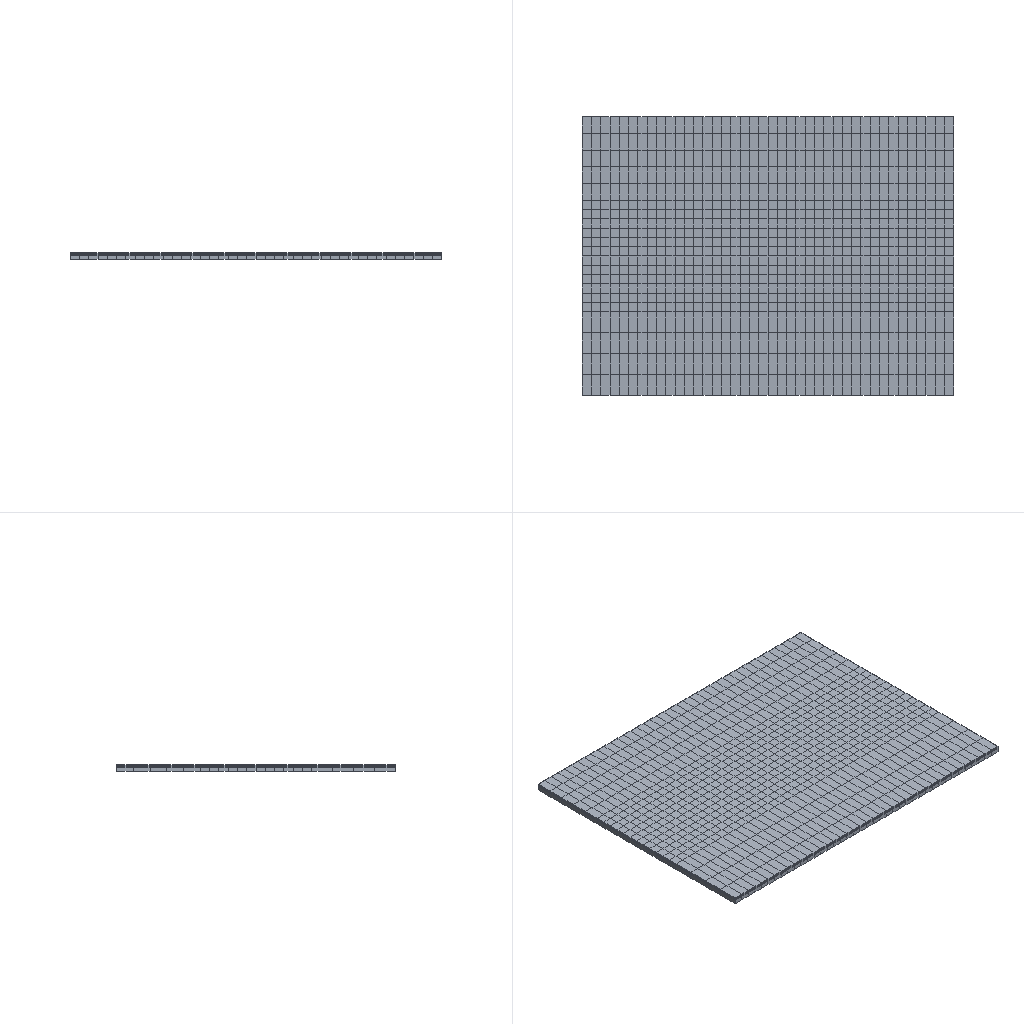Simulation study | abaqus
Set-up summary:
category,name,step,type,value,unit,region
solver,abaqus
solver,version,,,Abaqus/Explicit 3DEXPERIENCE R2017x
units,not stated in the deck,,not stated
analysis,deck,,transient,transient
load_step,Step-1,Step-1,transient
load_step,requested,,,1
mesh,nodes,,,10320
mesh,elements,,,9187
element_type,R3D3,,rigid,164
element_type,R3D4,,rigid,4823
element_type,C3D8R,,solid,4200
load,load commands in deck,,count,2
bc,support commands in deck,,count,7
material,MATERIAL-1,,in results
check,setup vs results,,match,"per instance, exact: element labels, types and connectivity; labels of the nodes the elements use; coordinates not compared"
Abaqus input file, long lists of numbers shortened:
*Heading
** Job name: Job-1 Model name: Job-2
** Generated by: Abaqus/CAE 2017
*Preprint, echo=NO, model=NO, history=NO, contact=NO
**
** PARTS
**
*Part, name=TOOL
*Node
      1,  0.9534, 0.04811, -0.7445
      2,  0.9637, 0.03641, -0.7418
** (4906 more lines like these left out)
*Element, type=R3D4
   1,    1,    2,  119,  126
   2,  126,  119,  120,  125
** (4821 more lines like these left out)
*Element, type=R3D3
2967,  252,   33, 1053
2972, 3534, 3528, 3533
** (162 more lines like these left out)
*Nset, nset=TOOL-RefPt_, internal
 4908,
*Nset, nset=TOOL-REFPT_, internal
 4908,
*Elset, elset=TOOL, generate
    1,  4987,     1
*End Part
**
*Part, name=WORK
*Node
      1,           8.,  -1.8, 0.09
      2,           8.,  -1.8,  0.15
** (5410 more lines like these left out)
*Element, type=C3D8R
   1,  120, 1549, 3307,  691,    1,   25,  625,   52
   2, 1549, 1550, 3308, 3307,   25,   26,  626,  625
** (4198 more lines like these left out)
*Nset, nset=SET-6, generate
    1,  5412,     1
*Elset, elset=SET-6, generate
    1,  4200,     1
** Section: Section-1-SET-6
*Solid Section, elset=SET-6, material=MATERIAL-1
,
*End Part
**
**
** ASSEMBLY
**
*Assembly, name=Assembly
**
*Instance, name=TOOL-1, part=TOOL
        -0.3,          -3.,          0.1
        -0.3,          -3.,          0.1,         -0.3,          -2.,          0.1,         180.
*End Instance
**
*Instance, name=WORK-1, part=WORK
*End Instance
**
*Nset, nset=SET-1, instance=WORK-1
    2,    3,    5,    6,   10,   12,   23,   24,   28,   29,   30,   31,   32,   33,   34,   35
   36,   37,   38,   56,   57,   58,   59,   60,   61,   62,   63,   64,   65,   66,  159,  160
** (55 more lines like these left out)
*Elset, elset=SET-1, instance=WORK-1
    4,    8,   12,   16,   20,   24,   28,   32,   36,   40,   44,   48,   52,   56,   60,   64
   68,   72,   76,   80,   84,   88,   92,   96,  100,  104,  108,  112,  116,  120,  124,  128
** (51 more lines like these left out)
*Nset, nset=SET-2, instance=TOOL-1
 4908,
*Nset, nset=SET-4, instance=WORK-1
   13,   14,   15,   17,   18,   19,   20,   21,  337,  338,  339,  340,  341,  342,  343,  344
  345,  346,  347,  348,  349,  350,  351,  355,  356,  357,  358,  359,  360,  361,  362,  363
** (55 more lines like these left out)
*Elset, elset=SET-4, instance=WORK-1, generate
 2721,  3560,     1
*Nset, nset=S_SET-3, instance=WORK-1
    1,    4,    7,    8,   14,   15,   18,   20,   42,   43,   44,   45,   46,   47,   48,   49
   50,   51,   52,   70,   71,   72,   73,   74,   75,   76,   77,   78,   79,   80,   81,   82
** (65 more lines like these left out)
*Elset, elset=S_SET-3, instance=WORK-1
    1,    5,    9,   13,   17,   21,   25,   29,   33,   37,   41,   45,   49,   53,   57,   61
   65,   69,   73,   77,   81,   85,   89,   93,   97,  101,  105,  109,  113,  117,  121,  125
** (63 more lines like these left out)
*Nset, nset=S_SET-3_CNS_, internal, instance=WORK-1
    1,    4,    7,    8,   14,   15,   18,   20,   42,   43,   44,   45,   46,   47,   48,   49
   50,   51,   52,   70,   71,   72,   73,   74,   75,   76,   77,   78,   79,   80,   81,   82
** (65 more lines like these left out)
*Elset, elset=_M_SURF-1_SPOS, internal, instance=TOOL-1
    1,    2,    3,    4,    5,    6,    7,    8,    9,   10,   11,   12,   13,   14,   15,   16
   17,   18,   19,   20,   21,   22,   23,   24,   25,   26,   27,   28,   29,   30,   31,   32
** (137 more lines like these left out)
*Surface, type=ELEMENT, name=M_SURF-1
_M_SURF-1_SPOS, SPOS
*Surface, type=NODE, name=S_SET-3_CNS__CNS_, internal
S_SET-3_CNS_, 1.
** Constraint: RigidBody-1
*Rigid Body, ref node=TOOL-1.TOOL-REFPT_, elset=TOOL-1.TOOL
*End Assembly
**
** MATERIALS
**
*Material, name=MATERIAL-1
*Density
 2e-10,
*Depvar, delete=1
      6,
*Hyperfoam, moduli=LONG TERM
 5.34, 1.87,  0.1
*User Defined Field
*Viscoelastic, frequency=PRONY
 0.3,  0.3, 0.01
**
** INTERACTION PROPERTIES
**
*Surface Interaction, name=INTPROP-1
*Friction
 0.2,
*Surface Behavior, pressure-overclosure=HARD
** ----------------------------------------------------------------
**
** STEP: Step-1
**
*Step, name=Step-1, nlgeom=YES
*Dynamic, Explicit
, 0.27
*Bulk Viscosity
0.06, 1.2
** Mass Scaling: Semi-Automatic
**               Whole Model
*Fixed Mass Scaling, factor=5000.
**
** BOUNDARY CONDITIONS
**
** Name: Disp-BC-1 Type: 对称/反对称/完全固定
*Boundary
SET-4, ENCASTRE
** Name: Vel-BC-1 Type: 速度/角速度
*Boundary, type=VELOCITY
SET-2, 1, 1, 30.
** Name: Vel-BC-2 Type: 速度/角速度
*Boundary, type=VELOCITY
SET-2, 2, 2
** Name: Vel-BC-3 Type: 速度/角速度
*Boundary, type=VELOCITY
SET-2, 3, 3
** Name: Vel-BC-4 Type: 速度/角速度
*Boundary, type=VELOCITY
SET-2, 4, 4
** Name: Vel-BC-5 Type: 速度/角速度
*Boundary, type=VELOCITY
SET-2, 5, 5
** Name: Vel-BC-6 Type: 速度/角速度
*Boundary, type=VELOCITY
SET-2, 6, 6, -28260.
**
** INTERACTIONS
**
** Interaction: INT-1-1
*Contact Pair, interaction=INTPROP-1, mechanical constraint=PENALTY, cpset=INT-1-1
M_SURF-1, S_SET-3_CNS__CNS_
** Interaction: Int-2
*Contact, op=NEW
*Contact Inclusions, ALL EXTERIOR
*Contact Property Assignment
 ,  , INTPROP-1
**
** OUTPUT REQUESTS
**
*Restart, write, number interval=1, time marks=NO
**
** FIELD OUTPUT: F-Output-1
**
*Output, field, number interval=100
*Node Output
A, RF, U, V
**
** FIELD OUTPUT: F-Output-3
**
*Element Output, directions=YES
FV, MFR, SDV, STATUS, UVARM
*Contact Output
CSTRESS,
**
** FIELD OUTPUT: F-Output-2
**
*Element Output, directions=YES
DAMAGEC, DAMAGET, E, LE, MISES, PE, PEEQ, PEEQVAVG, PEVAVG, S, SDEG, STATUS, SVAVG
**
** HISTORY OUTPUT: H-Output-1
**
*Output, history, variable=PRESELECT
*End Step
Results summary:
result,step,Step-1,completed,increments=176904 time=0.27/0.27
result,analysis,,,transient
result,last_loadstep,,,1
result,primary field,,,U
result,reaction total,,FX,-1.842,model units
result,reaction total,,FY,-1.849,model units
result,reaction total,,FZ,-0.03543,model units